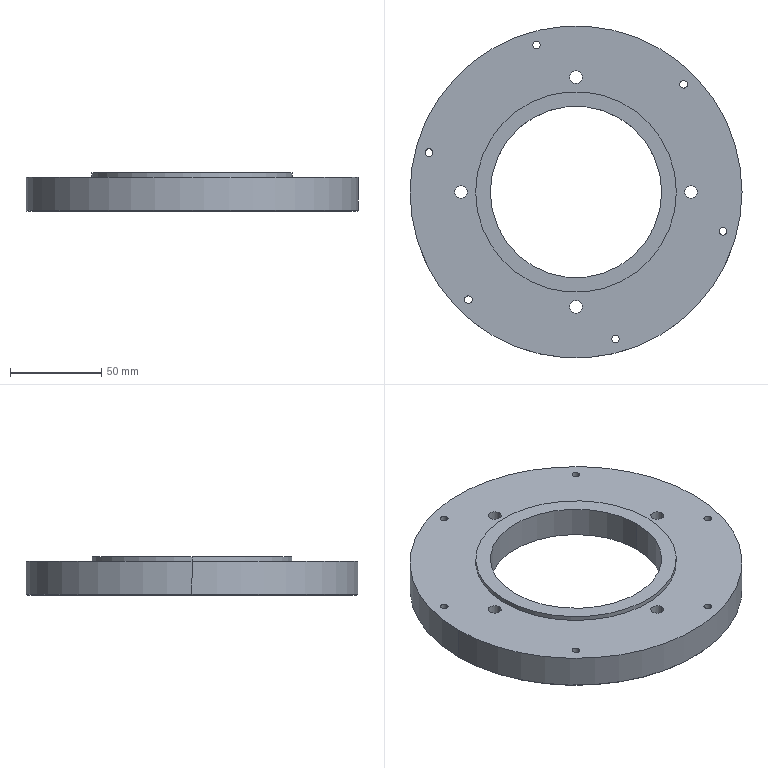Part | STEP file | Rear End Cover 2 | 1 solid | 46 faces | box 182 x 182 x 21 mm | volume 315087 mm3 | cylinder 36 | plane 8 | cone 2 | commonest cylinder face diameters 4.2 x12 7 x8 12 x8 94 x2 110 x2 145 x2
STEP:
#1=CARTESIAN_POINT('',(91.,0.,18.5));
#2=VERTEX_POINT('',#1);
#3=CARTESIAN_POINT('',(-91.,0.,18.5));
#4=VERTEX_POINT('',#3);
#5=CARTESIAN_POINT('',(0.,0.,18.5));
#6=DIRECTION('',(0.,0.,1.));
#7=DIRECTION('',(-1.,0.,0.));
#8=AXIS2_PLACEMENT_3D('',#5,#6,#7);
#9=CIRCLE('',#8,91.);
#10=EDGE_CURVE('',#2,#4,#9,.T.);
#11=ORIENTED_EDGE('',*,*,#10,.F.);
#12=CARTESIAN_POINT('',(91.,0.,0.5));
#13=VERTEX_POINT('',#12);
#14=CARTESIAN_POINT('',(91.,0.,275.887));
#15=DIRECTION('',(0.,0.,-1.));
#16=VECTOR('',#15,1000.);
#17=LINE('',#14,#16);
#18=EDGE_CURVE('',#2,#13,#17,.T.);
#19=ORIENTED_EDGE('',*,*,#18,.T.);
#20=CARTESIAN_POINT('',(-91.,0.,0.5));
#21=VERTEX_POINT('',#20);
#22=CARTESIAN_POINT('',(0.,0.,0.5));
#23=DIRECTION('',(0.,0.,1.));
#24=DIRECTION('',(-1.,0.,0.));
#25=AXIS2_PLACEMENT_3D('',#22,#23,#24);
#26=CIRCLE('',#25,91.);
#27=EDGE_CURVE('',#13,#21,#26,.T.);
#28=ORIENTED_EDGE('',*,*,#27,.T.);
#29=CARTESIAN_POINT('',(-91.,0.,275.887));
#30=DIRECTION('',(0.,0.,-1.));
#31=VECTOR('',#30,1000.);
#32=LINE('',#29,#31);
#33=EDGE_CURVE('',#4,#21,#32,.T.);
#34=ORIENTED_EDGE('',*,*,#33,.F.);
#35=EDGE_LOOP('',(#11,#19,#28,#34));
#36=FACE_OUTER_BOUND('',#35,.T.);
#37=CARTESIAN_POINT('',(0.,0.,275.887));
#38=DIRECTION('',(0.,0.,-1.));
#39=DIRECTION('',(-1.,0.,0.));
#40=AXIS2_PLACEMENT_3D('',#37,#38,#39);
#41=CYLINDRICAL_SURFACE('',#40,91.);
#42=ADVANCED_FACE('',(#36),#41,.T.);
#43=CARTESIAN_POINT('',(-55.,0.,21.));
#44=VERTEX_POINT('',#43);
#45=CARTESIAN_POINT('',(55.,0.,21.));
#46=VERTEX_POINT('',#45);
#47=CARTESIAN_POINT('',(0.,0.,21.));
#48=DIRECTION('',(0.,0.,-1.));
#49=DIRECTION('',(-1.,0.,0.));
#50=AXIS2_PLACEMENT_3D('',#47,#48,#49);
#51=CIRCLE('',#50,55.);
#52=EDGE_CURVE('',#44,#46,#51,.T.);
#53=ORIENTED_EDGE('',*,*,#52,.T.);
#54=CARTESIAN_POINT('',(55.,0.,18.5));
#55=VERTEX_POINT('',#54);
#56=CARTESIAN_POINT('',(55.,0.,21.));
#57=DIRECTION('',(0.,0.,-1.));
#58=VECTOR('',#57,1000.);
#59=LINE('',#56,#58);
#60=EDGE_CURVE('',#46,#55,#59,.T.);
#61=ORIENTED_EDGE('',*,*,#60,.T.);
#62=CARTESIAN_POINT('',(-55.,0.,18.5));
#63=VERTEX_POINT('',#62);
#64=CARTESIAN_POINT('',(0.,0.,18.5));
#65=DIRECTION('',(0.,0.,-1.));
#66=DIRECTION('',(-1.,0.,0.));
#67=AXIS2_PLACEMENT_3D('',#64,#65,#66);
#68=CIRCLE('',#67,55.);
#69=EDGE_CURVE('',#63,#55,#68,.T.);
#70=ORIENTED_EDGE('',*,*,#69,.F.);
#71=CARTESIAN_POINT('',(-55.,0.,21.));
#72=DIRECTION('',(0.,0.,-1.));
#73=VECTOR('',#72,1000.);
#74=LINE('',#71,#73);
#75=EDGE_CURVE('',#44,#63,#74,.T.);
#76=ORIENTED_EDGE('',*,*,#75,.F.);
#77=EDGE_LOOP('',(#53,#61,#70,#76));
#78=FACE_OUTER_BOUND('',#77,.T.);
#79=CARTESIAN_POINT('',(0.,0.,21.));
#80=DIRECTION('',(0.,0.,-1.));
#81=DIRECTION('',(-1.,0.,0.));
#82=AXIS2_PLACEMENT_3D('',#79,#80,#81);
#83=CYLINDRICAL_SURFACE('',#82,55.);
#84=ADVANCED_FACE('',(#78),#83,.T.);
#85=CARTESIAN_POINT('',(-3.5,63.,11.));
#86=VERTEX_POINT('',#85);
#87=CARTESIAN_POINT('',(3.5,63.,11.));
#88=VERTEX_POINT('',#87);
#89=CARTESIAN_POINT('',(0.,63.,11.));
#90=DIRECTION('',(0.,0.,1.));
#91=DIRECTION('',(1.,0.,0.));
#92=AXIS2_PLACEMENT_3D('',#89,#90,#91);
#93=CIRCLE('',#92,3.5);
#94=EDGE_CURVE('',#86,#88,#93,.T.);
#95=ORIENTED_EDGE('',*,*,#94,.F.);
#96=CARTESIAN_POINT('',(-3.5,63.,18.5));
#97=VERTEX_POINT('',#96);
#98=CARTESIAN_POINT('',(-3.5,63.,0.));
#99=DIRECTION('',(0.,0.,1.));
#100=VECTOR('',#99,1000.);
#101=LINE('',#98,#100);
#102=EDGE_CURVE('',#86,#97,#101,.T.);
#103=ORIENTED_EDGE('',*,*,#102,.T.);
#104=CARTESIAN_POINT('',(3.5,63.,18.5));
#105=VERTEX_POINT('',#104);
#106=CARTESIAN_POINT('',(0.,63.,18.5));
#107=DIRECTION('',(0.,0.,-1.));
#108=DIRECTION('',(1.,0.,0.));
#109=AXIS2_PLACEMENT_3D('',#106,#107,#108);
#110=CIRCLE('',#109,3.5);
#111=EDGE_CURVE('',#105,#97,#110,.T.);
#112=ORIENTED_EDGE('',*,*,#111,.F.);
#113=CARTESIAN_POINT('',(3.5,63.,0.));
#114=DIRECTION('',(0.,0.,1.));
#115=VECTOR('',#114,1000.);
#116=LINE('',#113,#115);
#117=EDGE_CURVE('',#88,#105,#116,.T.);
#118=ORIENTED_EDGE('',*,*,#117,.F.);
#119=EDGE_LOOP('',(#95,#103,#112,#118));
#120=FACE_OUTER_BOUND('',#119,.T.);
#121=CARTESIAN_POINT('',(0.,63.,0.));
#122=DIRECTION('',(0.,0.,1.));
#123=DIRECTION('',(1.,0.,0.));
#124=AXIS2_PLACEMENT_3D('',#121,#122,#123);
#125=CYLINDRICAL_SURFACE('',#124,3.5);
#126=ADVANCED_FACE('',(#120),#125,.F.);
#127=CARTESIAN_POINT('',(59.5,0.,11.));
#128=VERTEX_POINT('',#127);
#129=CARTESIAN_POINT('',(66.5,0.,11.));
#130=VERTEX_POINT('',#129);
#131=CARTESIAN_POINT('',(63.,0.,11.));
#132=DIRECTION('',(0.,0.,1.));
#133=DIRECTION('',(1.,0.,0.));
#134=AXIS2_PLACEMENT_3D('',#131,#132,#133);
#135=CIRCLE('',#134,3.5);
#136=EDGE_CURVE('',#128,#130,#135,.T.);
#137=ORIENTED_EDGE('',*,*,#136,.F.);
#138=CARTESIAN_POINT('',(59.5,0.,18.5));
#139=VERTEX_POINT('',#138);
#140=CARTESIAN_POINT('',(59.5,0.,0.));
#141=DIRECTION('',(0.,0.,1.));
#142=VECTOR('',#141,1000.);
#143=LINE('',#140,#142);
#144=EDGE_CURVE('',#128,#139,#143,.T.);
#145=ORIENTED_EDGE('',*,*,#144,.T.);
#146=CARTESIAN_POINT('',(66.5,0.,18.5));
#147=VERTEX_POINT('',#146);
#148=CARTESIAN_POINT('',(63.,0.,18.5));
#149=DIRECTION('',(0.,0.,-1.));
#150=DIRECTION('',(1.,0.,0.));
#151=AXIS2_PLACEMENT_3D('',#148,#149,#150);
#152=CIRCLE('',#151,3.5);
#153=EDGE_CURVE('',#147,#139,#152,.T.);
#154=ORIENTED_EDGE('',*,*,#153,.F.);
#155=CARTESIAN_POINT('',(66.5,0.,0.));
#156=DIRECTION('',(0.,0.,1.));
#157=VECTOR('',#156,1000.);
#158=LINE('',#155,#157);
#159=EDGE_CURVE('',#130,#147,#158,.T.);
#160=ORIENTED_EDGE('',*,*,#159,.F.);
#161=EDGE_LOOP('',(#137,#145,#154,#160));
#162=FACE_OUTER_BOUND('',#161,.T.);
#163=CARTESIAN_POINT('',(63.,0.,0.));
#164=DIRECTION('',(0.,0.,1.));
#165=DIRECTION('',(1.,0.,0.));
#166=AXIS2_PLACEMENT_3D('',#163,#164,#165);
#167=CYLINDRICAL_SURFACE('',#166,3.5);
#168=ADVANCED_FACE('',(#162),#167,.F.);
#169=CARTESIAN_POINT('',(-3.5,-63.,11.));
#170=VERTEX_POINT('',#169);
#171=CARTESIAN_POINT('',(3.5,-63.,11.));
#172=VERTEX_POINT('',#171);
#173=CARTESIAN_POINT('',(0.,-63.,11.));
#174=DIRECTION('',(0.,0.,1.));
#175=DIRECTION('',(1.,0.,0.));
#176=AXIS2_PLACEMENT_3D('',#173,#174,#175);
#177=CIRCLE('',#176,3.5);
#178=EDGE_CURVE('',#170,#172,#177,.T.);
#179=ORIENTED_EDGE('',*,*,#178,.F.);
#180=CARTESIAN_POINT('',(-3.5,-63.,18.5));
#181=VERTEX_POINT('',#180);
#182=CARTESIAN_POINT('',(-3.5,-63.,0.));
#183=DIRECTION('',(0.,0.,1.));
#184=VECTOR('',#183,1000.);
#185=LINE('',#182,#184);
#186=EDGE_CURVE('',#170,#181,#185,.T.);
#187=ORIENTED_EDGE('',*,*,#186,.T.);
#188=CARTESIAN_POINT('',(3.5,-63.,18.5));
#189=VERTEX_POINT('',#188);
#190=CARTESIAN_POINT('',(0.,-63.,18.5));
#191=DIRECTION('',(0.,0.,-1.));
#192=DIRECTION('',(1.,0.,0.));
#193=AXIS2_PLACEMENT_3D('',#190,#191,#192);
#194=CIRCLE('',#193,3.5);
#195=EDGE_CURVE('',#189,#181,#194,.T.);
#196=ORIENTED_EDGE('',*,*,#195,.F.);
#197=CARTESIAN_POINT('',(3.5,-63.,0.));
#198=DIRECTION('',(0.,0.,1.));
#199=VECTOR('',#198,1000.);
#200=LINE('',#197,#199);
#201=EDGE_CURVE('',#172,#189,#200,.T.);
#202=ORIENTED_EDGE('',*,*,#201,.F.);
#203=EDGE_LOOP('',(#179,#187,#196,#202));
#204=FACE_OUTER_BOUND('',#203,.T.);
#205=CARTESIAN_POINT('',(0.,-63.,0.));
#206=DIRECTION('',(0.,0.,1.));
#207=DIRECTION('',(1.,0.,0.));
#208=AXIS2_PLACEMENT_3D('',#205,#206,#207);
#209=CYLINDRICAL_SURFACE('',#208,3.5);
#210=ADVANCED_FACE('',(#204),#209,.F.);
#211=CARTESIAN_POINT('',(-66.5,0.,11.));
#212=VERTEX_POINT('',#211);
#213=CARTESIAN_POINT('',(-59.5,0.,11.));
#214=VERTEX_POINT('',#213);
#215=CARTESIAN_POINT('',(-63.,0.,11.));
#216=DIRECTION('',(0.,0.,1.));
#217=DIRECTION('',(1.,0.,0.));
#218=AXIS2_PLACEMENT_3D('',#215,#216,#217);
#219=CIRCLE('',#218,3.5);
#220=EDGE_CURVE('',#212,#214,#219,.T.);
#221=ORIENTED_EDGE('',*,*,#220,.F.);
#222=CARTESIAN_POINT('',(-66.5,0.,18.5));
#223=VERTEX_POINT('',#222);
#224=CARTESIAN_POINT('',(-66.5,0.,0.));
#225=DIRECTION('',(0.,0.,1.));
#226=VECTOR('',#225,1000.);
#227=LINE('',#224,#226);
#228=EDGE_CURVE('',#212,#223,#227,.T.);
#229=ORIENTED_EDGE('',*,*,#228,.T.);
#230=CARTESIAN_POINT('',(-59.5,0.,18.5));
#231=VERTEX_POINT('',#230);
#232=CARTESIAN_POINT('',(-63.,0.,18.5));
#233=DIRECTION('',(0.,0.,-1.));
#234=DIRECTION('',(1.,0.,0.));
#235=AXIS2_PLACEMENT_3D('',#232,#233,#234);
#236=CIRCLE('',#235,3.5);
#237=EDGE_CURVE('',#231,#223,#236,.T.);
#238=ORIENTED_EDGE('',*,*,#237,.F.);
#239=CARTESIAN_POINT('',(-59.5,0.,0.));
#240=DIRECTION('',(0.,0.,1.));
#241=VECTOR('',#240,1000.);
#242=LINE('',#239,#241);
#243=EDGE_CURVE('',#214,#231,#242,.T.);
#244=ORIENTED_EDGE('',*,*,#243,.F.);
#245=EDGE_LOOP('',(#221,#229,#238,#244));
#246=FACE_OUTER_BOUND('',#245,.T.);
#247=CARTESIAN_POINT('',(-63.,0.,0.));
#248=DIRECTION('',(0.,0.,1.));
#249=DIRECTION('',(1.,0.,0.));
#250=AXIS2_PLACEMENT_3D('',#247,#248,#249);
#251=CYLINDRICAL_SURFACE('',#250,3.5);
#252=ADVANCED_FACE('',(#246),#251,.F.);
#253=CARTESIAN_POINT('',(61.101,59.001,18.5));
#254=VERTEX_POINT('',#253);
#255=CARTESIAN_POINT('',(56.901,59.001,18.5));
#256=VERTEX_POINT('',#255);
#257=CARTESIAN_POINT('',(59.001,59.001,18.5));
#258=DIRECTION('',(0.,0.,-1.));
#259=DIRECTION('',(-1.,0.,0.));
#260=AXIS2_PLACEMENT_3D('',#257,#258,#259);
#261=CIRCLE('',#260,2.1);
#262=EDGE_CURVE('',#254,#256,#261,.T.);
#263=ORIENTED_EDGE('',*,*,#262,.F.);
#264=CARTESIAN_POINT('',(61.101,59.001,0.));
#265=VERTEX_POINT('',#264);
#266=CARTESIAN_POINT('',(61.101,59.001,21.));
#267=DIRECTION('',(0.,0.,-1.));
#268=VECTOR('',#267,1000.);
#269=LINE('',#266,#268);
#270=EDGE_CURVE('',#254,#265,#269,.T.);
#271=ORIENTED_EDGE('',*,*,#270,.T.);
#272=CARTESIAN_POINT('',(56.901,59.001,0.));
#273=VERTEX_POINT('',#272);
#274=CARTESIAN_POINT('',(59.001,59.001,0.));
#275=DIRECTION('',(0.,0.,1.));
#276=DIRECTION('',(-1.,0.,0.));
#277=AXIS2_PLACEMENT_3D('',#274,#275,#276);
#278=CIRCLE('',#277,2.1);
#279=EDGE_CURVE('',#273,#265,#278,.T.);
#280=ORIENTED_EDGE('',*,*,#279,.F.);
#281=CARTESIAN_POINT('',(56.901,59.001,21.));
#282=DIRECTION('',(0.,0.,-1.));
#283=VECTOR('',#282,1000.);
#284=LINE('',#281,#283);
#285=EDGE_CURVE('',#256,#273,#284,.T.);
#286=ORIENTED_EDGE('',*,*,#285,.F.);
#287=EDGE_LOOP('',(#263,#271,#280,#286));
#288=FACE_OUTER_BOUND('',#287,.T.);
#289=CARTESIAN_POINT('',(59.001,59.001,21.));
#290=DIRECTION('',(0.,0.,-1.));
#291=DIRECTION('',(-1.,0.,0.));
#292=AXIS2_PLACEMENT_3D('',#289,#290,#291);
#293=CYLINDRICAL_SURFACE('',#292,2.1);
#294=ADVANCED_FACE('',(#288),#293,.F.);
#295=CARTESIAN_POINT('',(-19.496,80.597,18.5));
#296=VERTEX_POINT('',#295);
#297=CARTESIAN_POINT('',(-23.696,80.597,18.5));
#298=VERTEX_POINT('',#297);
#299=CARTESIAN_POINT('',(-21.596,80.597,18.5));
#300=DIRECTION('',(0.,0.,-1.));
#301=DIRECTION('',(-1.,0.,0.));
#302=AXIS2_PLACEMENT_3D('',#299,#300,#301);
#303=CIRCLE('',#302,2.1);
#304=EDGE_CURVE('',#296,#298,#303,.T.);
#305=ORIENTED_EDGE('',*,*,#304,.F.);
#306=CARTESIAN_POINT('',(-19.496,80.597,0.));
#307=VERTEX_POINT('',#306);
#308=CARTESIAN_POINT('',(-19.496,80.597,21.));
#309=DIRECTION('',(0.,0.,-1.));
#310=VECTOR('',#309,1000.);
#311=LINE('',#308,#310);
#312=EDGE_CURVE('',#296,#307,#311,.T.);
#313=ORIENTED_EDGE('',*,*,#312,.T.);
#314=CARTESIAN_POINT('',(-23.696,80.597,0.));
#315=VERTEX_POINT('',#314);
#316=CARTESIAN_POINT('',(-21.596,80.597,0.));
#317=DIRECTION('',(0.,0.,1.));
#318=DIRECTION('',(-1.,0.,0.));
#319=AXIS2_PLACEMENT_3D('',#316,#317,#318);
#320=CIRCLE('',#319,2.1);
#321=EDGE_CURVE('',#315,#307,#320,.T.);
#322=ORIENTED_EDGE('',*,*,#321,.F.);
#323=CARTESIAN_POINT('',(-23.696,80.597,21.));
#324=DIRECTION('',(0.,0.,-1.));
#325=VECTOR('',#324,1000.);
#326=LINE('',#323,#325);
#327=EDGE_CURVE('',#298,#315,#326,.T.);
#328=ORIENTED_EDGE('',*,*,#327,.F.);
#329=EDGE_LOOP('',(#305,#313,#322,#328));
#330=FACE_OUTER_BOUND('',#329,.T.);
#331=CARTESIAN_POINT('',(-21.596,80.597,21.));
#332=DIRECTION('',(0.,0.,-1.));
#333=DIRECTION('',(-1.,0.,0.));
#334=AXIS2_PLACEMENT_3D('',#331,#332,#333);
#335=CYLINDRICAL_SURFACE('',#334,2.1);
#336=ADVANCED_FACE('',(#330),#335,.F.);
#337=CARTESIAN_POINT('',(-78.497,21.596,18.5));
#338=VERTEX_POINT('',#337);
#339=CARTESIAN_POINT('',(-82.697,21.596,18.5));
#340=VERTEX_POINT('',#339);
#341=CARTESIAN_POINT('',(-80.597,21.596,18.5));
#342=DIRECTION('',(0.,0.,-1.));
#343=DIRECTION('',(-1.,0.,0.));
#344=AXIS2_PLACEMENT_3D('',#341,#342,#343);
#345=CIRCLE('',#344,2.1);
#346=EDGE_CURVE('',#338,#340,#345,.T.);
#347=ORIENTED_EDGE('',*,*,#346,.F.);
#348=CARTESIAN_POINT('',(-78.497,21.596,0.));
#349=VERTEX_POINT('',#348);
#350=CARTESIAN_POINT('',(-78.497,21.596,21.));
#351=DIRECTION('',(0.,0.,-1.));
#352=VECTOR('',#351,1000.);
#353=LINE('',#350,#352);
#354=EDGE_CURVE('',#338,#349,#353,.T.);
#355=ORIENTED_EDGE('',*,*,#354,.T.);
#356=CARTESIAN_POINT('',(-82.697,21.596,0.));
#357=VERTEX_POINT('',#356);
#358=CARTESIAN_POINT('',(-80.597,21.596,0.));
#359=DIRECTION('',(0.,0.,1.));
#360=DIRECTION('',(-1.,0.,0.));
#361=AXIS2_PLACEMENT_3D('',#358,#359,#360);
#362=CIRCLE('',#361,2.1);
#363=EDGE_CURVE('',#357,#349,#362,.T.);
#364=ORIENTED_EDGE('',*,*,#363,.F.);
#365=CARTESIAN_POINT('',(-82.697,21.596,21.));
#366=DIRECTION('',(0.,0.,-1.));
#367=VECTOR('',#366,1000.);
#368=LINE('',#365,#367);
#369=EDGE_CURVE('',#340,#357,#368,.T.);
#370=ORIENTED_EDGE('',*,*,#369,.F.);
#371=EDGE_LOOP('',(#347,#355,#364,#370));
#372=FACE_OUTER_BOUND('',#371,.T.);
#373=CARTESIAN_POINT('',(-80.597,21.596,21.));
#374=DIRECTION('',(0.,0.,-1.));
#375=DIRECTION('',(-1.,0.,0.));
#376=AXIS2_PLACEMENT_3D('',#373,#374,#375);
#377=CYLINDRICAL_SURFACE('',#376,2.1);
#378=ADVANCED_FACE('',(#372),#377,.F.);
#379=CARTESIAN_POINT('',(-56.901,-59.001,18.5));
#380=VERTEX_POINT('',#379);
#381=CARTESIAN_POINT('',(-61.101,-59.001,18.5));
#382=VERTEX_POINT('',#381);
#383=CARTESIAN_POINT('',(-59.001,-59.001,18.5));
#384=DIRECTION('',(0.,0.,-1.));
#385=DIRECTION('',(-1.,0.,0.));
#386=AXIS2_PLACEMENT_3D('',#383,#384,#385);
#387=CIRCLE('',#386,2.1);
#388=EDGE_CURVE('',#380,#382,#387,.T.);
#389=ORIENTED_EDGE('',*,*,#388,.F.);
#390=CARTESIAN_POINT('',(-56.901,-59.001,0.));
#391=VERTEX_POINT('',#390);
#392=CARTESIAN_POINT('',(-56.901,-59.001,21.));
#393=DIRECTION('',(0.,0.,-1.));
#394=VECTOR('',#393,1000.);
#395=LINE('',#392,#394);
#396=EDGE_CURVE('',#380,#391,#395,.T.);
#397=ORIENTED_EDGE('',*,*,#396,.T.);
#398=CARTESIAN_POINT('',(-61.101,-59.001,0.));
#399=VERTEX_POINT('',#398);
#400=CARTESIAN_POINT('',(-59.001,-59.001,0.));
#401=DIRECTION('',(0.,0.,1.));
#402=DIRECTION('',(-1.,0.,0.));
#403=AXIS2_PLACEMENT_3D('',#400,#401,#402);
#404=CIRCLE('',#403,2.1);
#405=EDGE_CURVE('',#399,#391,#404,.T.);
#406=ORIENTED_EDGE('',*,*,#405,.F.);
#407=CARTESIAN_POINT('',(-61.101,-59.001,21.));
#408=DIRECTION('',(0.,0.,-1.));
#409=VECTOR('',#408,1000.);
#410=LINE('',#407,#409);
#411=EDGE_CURVE('',#382,#399,#410,.T.);
#412=ORIENTED_EDGE('',*,*,#411,.F.);
#413=EDGE_LOOP('',(#389,#397,#406,#412));
#414=FACE_OUTER_BOUND('',#413,.T.);
#415=CARTESIAN_POINT('',(-59.001,-59.001,21.));
#416=DIRECTION('',(0.,0.,-1.));
#417=DIRECTION('',(-1.,0.,0.));
#418=AXIS2_PLACEMENT_3D('',#415,#416,#417);
#419=CYLINDRICAL_SURFACE('',#418,2.1);
#420=ADVANCED_FACE('',(#414),#419,.F.);
#421=CARTESIAN_POINT('',(23.696,-80.597,18.5));
#422=VERTEX_POINT('',#421);
#423=CARTESIAN_POINT('',(19.496,-80.597,18.5));
#424=VERTEX_POINT('',#423);
#425=CARTESIAN_POINT('',(21.596,-80.597,18.5));
#426=DIRECTION('',(0.,0.,-1.));
#427=DIRECTION('',(-1.,0.,0.));
#428=AXIS2_PLACEMENT_3D('',#425,#426,#427);
#429=CIRCLE('',#428,2.1);
#430=EDGE_CURVE('',#422,#424,#429,.T.);
#431=ORIENTED_EDGE('',*,*,#430,.F.);
#432=CARTESIAN_POINT('',(23.696,-80.597,0.));
#433=VERTEX_POINT('',#432);
#434=CARTESIAN_POINT('',(23.696,-80.597,21.));
#435=DIRECTION('',(0.,0.,-1.));
#436=VECTOR('',#435,1000.);
#437=LINE('',#434,#436);
#438=EDGE_CURVE('',#422,#433,#437,.T.);
#439=ORIENTED_EDGE('',*,*,#438,.T.);
#440=CARTESIAN_POINT('',(19.496,-80.597,0.));
#441=VERTEX_POINT('',#440);
#442=CARTESIAN_POINT('',(21.596,-80.597,0.));
#443=DIRECTION('',(0.,0.,1.));
#444=DIRECTION('',(-1.,0.,0.));
#445=AXIS2_PLACEMENT_3D('',#442,#443,#444);
#446=CIRCLE('',#445,2.1);
#447=EDGE_CURVE('',#441,#433,#446,.T.);
#448=ORIENTED_EDGE('',*,*,#447,.F.);
#449=CARTESIAN_POINT('',(19.496,-80.597,21.));
#450=DIRECTION('',(0.,0.,-1.));
#451=VECTOR('',#450,1000.);
#452=LINE('',#449,#451);
#453=EDGE_CURVE('',#424,#441,#452,.T.);
#454=ORIENTED_EDGE('',*,*,#453,.F.);
#455=EDGE_LOOP('',(#431,#439,#448,#454));
#456=FACE_OUTER_BOUND('',#455,.T.);
#457=CARTESIAN_POINT('',(21.596,-80.597,21.));
#458=DIRECTION('',(0.,0.,-1.));
#459=DIRECTION('',(-1.,0.,0.));
#460=AXIS2_PLACEMENT_3D('',#457,#458,#459);
#461=CYLINDRICAL_SURFACE('',#460,2.1);
#462=ADVANCED_FACE('',(#456),#461,.F.);
#463=CARTESIAN_POINT('',(82.697,-21.596,18.5));
#464=VERTEX_POINT('',#463);
#465=CARTESIAN_POINT('',(78.497,-21.596,18.5));
#466=VERTEX_POINT('',#465);
#467=CARTESIAN_POINT('',(80.597,-21.596,18.5));
#468=DIRECTION('',(0.,0.,-1.));
#469=DIRECTION('',(-1.,0.,0.));
#470=AXIS2_PLACEMENT_3D('',#467,#468,#469);
#471=CIRCLE('',#470,2.1);
#472=EDGE_CURVE('',#464,#466,#471,.T.);
#473=ORIENTED_EDGE('',*,*,#472,.F.);
#474=CARTESIAN_POINT('',(82.697,-21.596,0.));
#475=VERTEX_POINT('',#474);
#476=CARTESIAN_POINT('',(82.697,-21.596,21.));
#477=DIRECTION('',(0.,0.,-1.));
#478=VECTOR('',#477,1000.);
#479=LINE('',#476,#478);
#480=EDGE_CURVE('',#464,#475,#479,.T.);
#481=ORIENTED_EDGE('',*,*,#480,.T.);
#482=CARTESIAN_POINT('',(78.497,-21.596,0.));
#483=VERTEX_POINT('',#482);
#484=CARTESIAN_POINT('',(80.597,-21.596,0.));
#485=DIRECTION('',(0.,0.,1.));
#486=DIRECTION('',(-1.,0.,0.));
#487=AXIS2_PLACEMENT_3D('',#484,#485,#486);
#488=CIRCLE('',#487,2.1);
#489=EDGE_CURVE('',#483,#475,#488,.T.);
#490=ORIENTED_EDGE('',*,*,#489,.F.);
#491=CARTESIAN_POINT('',(78.497,-21.596,21.));
#492=DIRECTION('',(0.,0.,-1.));
#493=VECTOR('',#492,1000.);
#494=LINE('',#491,#493);
#495=EDGE_CURVE('',#466,#483,#494,.T.);
#496=ORIENTED_EDGE('',*,*,#495,.F.);
#497=EDGE_LOOP('',(#473,#481,#490,#496));
#498=FACE_OUTER_BOUND('',#497,.T.);
#499=CARTESIAN_POINT('',(80.597,-21.596,21.));
#500=DIRECTION('',(0.,0.,-1.));
#501=DIRECTION('',(-1.,0.,0.));
#502=AXIS2_PLACEMENT_3D('',#499,#500,#501);
#503=CYLINDRICAL_SURFACE('',#502,2.1);
#504=ADVANCED_FACE('',(#498),#503,.F.);
#505=CARTESIAN_POINT('',(90.5,0.,0.));
#506=VERTEX_POINT('',#505);
#507=CARTESIAN_POINT('',(-90.5,0.,0.));
#508=VERTEX_POINT('',#507);
#509=CARTESIAN_POINT('',(0.,0.,0.));
#510=DIRECTION('',(0.,0.,1.));
#511=DIRECTION('',(1.,0.,0.));
#512=AXIS2_PLACEMENT_3D('',#509,#510,#511);
#513=CIRCLE('',#512,90.5);
#514=EDGE_CURVE('',#506,#508,#513,.T.);
#515=ORIENTED_EDGE('',*,*,#514,.T.);
#516=CARTESIAN_POINT('',(-91.,0.,0.5));
#517=DIRECTION('',(-0.7071,0.,0.7071));
#518=VECTOR('',#517,1000.);
#519=LINE('',#516,#518);
#520=EDGE_CURVE('',#508,#21,#519,.T.);
#521=ORIENTED_EDGE('',*,*,#520,.T.);
#522=ORIENTED_EDGE('',*,*,#27,.F.);
#523=CARTESIAN_POINT('',(91.,0.,0.5));
#524=DIRECTION('',(0.7071,0.,0.7071));
#525=VECTOR('',#524,1000.);
#526=LINE('',#523,#525);
#527=EDGE_CURVE('',#506,#13,#526,.T.);
#528=ORIENTED_EDGE('',*,*,#527,.F.);
#529=EDGE_LOOP('',(#515,#521,#522,#528));
#530=FACE_OUTER_BOUND('',#529,.T.);
#531=CARTESIAN_POINT('',(0.,0.,0.5));
#532=DIRECTION('',(0.,0.,1.));
#533=DIRECTION('',(1.,0.,0.));
#534=AXIS2_PLACEMENT_3D('',#531,#532,#533);
#535=CONICAL_SURFACE('',#534,91.,0.7854);
#536=ADVANCED_FACE('',(#530),#535,.T.);
#537=CARTESIAN_POINT('',(47.,0.,21.));
#538=VERTEX_POINT('',#537);
#539=CARTESIAN_POINT('',(-47.,0.,21.));
#540=VERTEX_POINT('',#539);
#541=CARTESIAN_POINT('',(0.,0.,21.));
#542=DIRECTION('',(0.,0.,-1.));
#543=DIRECTION('',(-1.,0.,0.));
#544=AXIS2_PLACEMENT_3D('',#541,#542,#543);
#545=CIRCLE('',#544,47.);
#546=EDGE_CURVE('',#538,#540,#545,.T.);
#547=ORIENTED_EDGE('',*,*,#546,.F.);
#548=CARTESIAN_POINT('',(47.,0.,4.));
#549=VERTEX_POINT('',#548);
#550=CARTESIAN_POINT('',(47.,0.,18.5));
#551=DIRECTION('',(0.,0.,-1.));
#552=VECTOR('',#551,1000.);
#553=LINE('',#550,#552);
#554=EDGE_CURVE('',#538,#549,#553,.T.);
#555=ORIENTED_EDGE('',*,*,#554,.T.);
#556=CARTESIAN_POINT('',(-47.,0.,4.));
#557=VERTEX_POINT('',#556);
#558=CARTESIAN_POINT('',(0.,0.,4.));
#559=DIRECTION('',(0.,0.,1.));
#560=DIRECTION('',(-1.,0.,0.));
#561=AXIS2_PLACEMENT_3D('',#558,#559,#560);
#562=CIRCLE('',#561,47.);
#563=EDGE_CURVE('',#557,#549,#562,.T.);
#564=ORIENTED_EDGE('',*,*,#563,.F.);
#565=CARTESIAN_POINT('',(-47.,0.,18.5));
#566=DIRECTION('',(0.,0.,-1.));
#567=VECTOR('',#566,1000.);
#568=LINE('',#565,#567);
#569=EDGE_CURVE('',#540,#557,#568,.T.);
#570=ORIENTED_EDGE('',*,*,#569,.F.);
#571=EDGE_LOOP('',(#547,#555,#564,#570));
#572=FACE_OUTER_BOUND('',#571,.T.);
#573=CARTESIAN_POINT('',(0.,0.,18.5));
#574=DIRECTION('',(0.,0.,-1.));
#575=DIRECTION('',(-1.,0.,0.));
#576=AXIS2_PLACEMENT_3D('',#573,#574,#575);
#577=CYLINDRICAL_SURFACE('',#576,47.);
#578=ADVANCED_FACE('',(#572),#577,.F.);
#579=CARTESIAN_POINT('',(6.,63.,11.));
#580=VERTEX_POINT('',#579);
#581=CARTESIAN_POINT('',(-6.,63.,11.));
#582=VERTEX_POINT('',#581);
#583=CARTESIAN_POINT('',(0.,63.,11.));
#584=DIRECTION('',(0.,0.,-1.));
#585=DIRECTION('',(-1.,0.,0.));
#586=AXIS2_PLACEMENT_3D('',#583,#584,#585);
#587=CIRCLE('',#586,6.);
#588=EDGE_CURVE('',#580,#582,#587,.T.);
#589=ORIENTED_EDGE('',*,*,#588,.F.);
#590=CARTESIAN_POINT('',(6.,63.,4.));
#591=VERTEX_POINT('',#590);
#592=CARTESIAN_POINT('',(6.,63.,11.));
#593=DIRECTION('',(0.,0.,-1.));
#594=VECTOR('',#593,1000.);
#595=LINE('',#592,#594);
#596=EDGE_CURVE('',#580,#591,#595,.T.);
#597=ORIENTED_EDGE('',*,*,#596,.T.);
#598=CARTESIAN_POINT('',(-6.,63.,4.));
#599=VERTEX_POINT('',#598);
#600=CARTESIAN_POINT('',(0.,63.,4.));
#601=DIRECTION('',(0.,0.,1.));
#602=DIRECTION('',(-1.,0.,0.));
#603=AXIS2_PLACEMENT_3D('',#600,#601,#602);
#604=CIRCLE('',#603,6.);
#605=EDGE_CURVE('',#599,#591,#604,.T.);
#606=ORIENTED_EDGE('',*,*,#605,.F.);
#607=CARTESIAN_POINT('',(-6.,63.,11.));
#608=DIRECTION('',(0.,0.,-1.));
#609=VECTOR('',#608,1000.);
#610=LINE('',#607,#609);
#611=EDGE_CURVE('',#582,#599,#610,.T.);
#612=ORIENTED_EDGE('',*,*,#611,.F.);
#613=EDGE_LOOP('',(#589,#597,#606,#612));
#614=FACE_OUTER_BOUND('',#613,.T.);
#615=CARTESIAN_POINT('',(0.,63.,11.));
#616=DIRECTION('',(0.,0.,-1.));
#617=DIRECTION('',(-1.,0.,0.));
#618=AXIS2_PLACEMENT_3D('',#615,#616,#617);
#619=CYLINDRICAL_SURFACE('',#618,6.);
#620=ADVANCED_FACE('',(#614),#619,.F.);
#621=CARTESIAN_POINT('',(69.,0.,11.));
#622=VERTEX_POINT('',#621);
#623=CARTESIAN_POINT('',(57.,0.,11.));
#624=VERTEX_POINT('',#623);
#625=CARTESIAN_POINT('',(63.,0.,11.));
#626=DIRECTION('',(0.,0.,-1.));
#627=DIRECTION('',(-1.,0.,0.));
#628=AXIS2_PLACEMENT_3D('',#625,#626,#627);
#629=CIRCLE('',#628,6.);
#630=EDGE_CURVE('',#622,#624,#629,.T.);
#631=ORIENTED_EDGE('',*,*,#630,.F.);
#632=CARTESIAN_POINT('',(69.,0.,4.));
#633=VERTEX_POINT('',#632);
#634=CARTESIAN_POINT('',(69.,0.,11.));
#635=DIRECTION('',(0.,0.,-1.));
#636=VECTOR('',#635,1000.);
#637=LINE('',#634,#636);
#638=EDGE_CURVE('',#622,#633,#637,.T.);
#639=ORIENTED_EDGE('',*,*,#638,.T.);
#640=CARTESIAN_POINT('',(57.,0.,4.));
#641=VERTEX_POINT('',#640);
#642=CARTESIAN_POINT('',(63.,0.,4.));
#643=DIRECTION('',(0.,0.,1.));
#644=DIRECTION('',(-1.,0.,0.));
#645=AXIS2_PLACEMENT_3D('',#642,#643,#644);
#646=CIRCLE('',#645,6.);
#647=EDGE_CURVE('',#641,#633,#646,.T.);
#648=ORIENTED_EDGE('',*,*,#647,.F.);
#649=CARTESIAN_POINT('',(57.,0.,11.));
#650=DIRECTION('',(0.,0.,-1.));
#651=VECTOR('',#650,1000.);
#652=LINE('',#649,#651);
#653=EDGE_CURVE('',#624,#641,#652,.T.);
#654=ORIENTED_EDGE('',*,*,#653,.F.);
#655=EDGE_LOOP('',(#631,#639,#648,#654));
#656=FACE_OUTER_BOUND('',#655,.T.);
#657=CARTESIAN_POINT('',(63.,0.,11.));
#658=DIRECTION('',(0.,0.,-1.));
#659=DIRECTION('',(-1.,0.,0.));
#660=AXIS2_PLACEMENT_3D('',#657,#658,#659);
#661=CYLINDRICAL_SURFACE('',#660,6.);
#662=ADVANCED_FACE('',(#656),#661,.F.);
#663=CARTESIAN_POINT('',(6.,-63.,11.));
#664=VERTEX_POINT('',#663);
#665=CARTESIAN_POINT('',(-6.,-63.,11.));
#666=VERTEX_POINT('',#665);
#667=CARTESIAN_POINT('',(0.,-63.,11.));
#668=DIRECTION('',(0.,0.,-1.));
#669=DIRECTION('',(-1.,0.,0.));
#670=AXIS2_PLACEMENT_3D('',#667,#668,#669);
#671=CIRCLE('',#670,6.);
#672=EDGE_CURVE('',#664,#666,#671,.T.);
#673=ORIENTED_EDGE('',*,*,#672,.F.);
#674=CARTESIAN_POINT('',(6.,-63.,4.));
#675=VERTEX_POINT('',#674);
#676=CARTESIAN_POINT('',(6.,-63.,11.));
#677=DIRECTION('',(0.,0.,-1.));
#678=VECTOR('',#677,1000.);
#679=LINE('',#676,#678);
#680=EDGE_CURVE('',#664,#675,#679,.T.);
#681=ORIENTED_EDGE('',*,*,#680,.T.);
#682=CARTESIAN_POINT('',(-6.,-63.,4.));
#683=VERTEX_POINT('',#682);
#684=CARTESIAN_POINT('',(0.,-63.,4.));
#685=DIRECTION('',(0.,0.,1.));
#686=DIRECTION('',(-1.,0.,0.));
#687=AXIS2_PLACEMENT_3D('',#684,#685,#686);
#688=CIRCLE('',#687,6.);
#689=EDGE_CURVE('',#683,#675,#688,.T.);
#690=ORIENTED_EDGE('',*,*,#689,.F.);
#691=CARTESIAN_POINT('',(-6.,-63.,11.));
#692=DIRECTION('',(0.,0.,-1.));
#693=VECTOR('',#692,1000.);
#694=LINE('',#691,#693);
#695=EDGE_CURVE('',#666,#683,#694,.T.);
#696=ORIENTED_EDGE('',*,*,#695,.F.);
#697=EDGE_LOOP('',(#673,#681,#690,#696));
#698=FACE_OUTER_BOUND('',#697,.T.);
#699=CARTESIAN_POINT('',(0.,-63.,11.));
#700=DIRECTION('',(0.,0.,-1.));
#701=DIRECTION('',(-1.,0.,0.));
#702=AXIS2_PLACEMENT_3D('',#699,#700,#701);
#703=CYLINDRICAL_SURFACE('',#702,6.);
#704=ADVANCED_FACE('',(#698),#703,.F.);
#705=CARTESIAN_POINT('',(-57.,0.,11.));
#706=VERTEX_POINT('',#705);
#707=CARTESIAN_POINT('',(-69.,0.,11.));
#708=VERTEX_POINT('',#707);
#709=CARTESIAN_POINT('',(-63.,0.,11.));
#710=DIRECTION('',(0.,0.,-1.));
#711=DIRECTION('',(-1.,0.,0.));
#712=AXIS2_PLACEMENT_3D('',#709,#710,#711);
#713=CIRCLE('',#712,6.);
#714=EDGE_CURVE('',#706,#708,#713,.T.);
#715=ORIENTED_EDGE('',*,*,#714,.F.);
#716=CARTESIAN_POINT('',(-57.,0.,4.));
#717=VERTEX_POINT('',#716);
#718=CARTESIAN_POINT('',(-57.,0.,11.));
#719=DIRECTION('',(0.,0.,-1.));
#720=VECTOR('',#719,1000.);
#721=LINE('',#718,#720);
#722=EDGE_CURVE('',#706,#717,#721,.T.);
#723=ORIENTED_EDGE('',*,*,#722,.T.);
#724=CARTESIAN_POINT('',(-69.,0.,4.));
#725=VERTEX_POINT('',#724);
#726=CARTESIAN_POINT('',(-63.,0.,4.));
#727=DIRECTION('',(0.,0.,1.));
#728=DIRECTION('',(-1.,0.,0.));
#729=AXIS2_PLACEMENT_3D('',#726,#727,#728);
#730=CIRCLE('',#729,6.);
#731=EDGE_CURVE('',#725,#717,#730,.T.);
#732=ORIENTED_EDGE('',*,*,#731,.F.);
#733=CARTESIAN_POINT('',(-69.,0.,11.));
#734=DIRECTION('',(0.,0.,-1.));
#735=VECTOR('',#734,1000.);
#736=LINE('',#733,#735);
#737=EDGE_CURVE('',#708,#725,#736,.T.);
#738=ORIENTED_EDGE('',*,*,#737,.F.);
#739=EDGE_LOOP('',(#715,#723,#732,#738));
#740=FACE_OUTER_BOUND('',#739,.T.);
#741=CARTESIAN_POINT('',(-63.,0.,11.));
#742=DIRECTION('',(0.,0.,-1.));
#743=DIRECTION('',(-1.,0.,0.));
#744=AXIS2_PLACEMENT_3D('',#741,#742,#743);
#745=CYLINDRICAL_SURFACE('',#744,6.);
#746=ADVANCED_FACE('',(#740),#745,.F.);
#747=CARTESIAN_POINT('',(72.5,0.,4.));
#748=VERTEX_POINT('',#747);
#749=CARTESIAN_POINT('',(-72.5,0.,4.));
#750=VERTEX_POINT('',#749);
#751=CARTESIAN_POINT('',(0.,0.,4.));
#752=DIRECTION('',(0.,0.,-1.));
#753=DIRECTION('',(-1.,0.,0.));
#754=AXIS2_PLACEMENT_3D('',#751,#752,#753);
#755=CIRCLE('',#754,72.5);
#756=EDGE_CURVE('',#748,#750,#755,.T.);
#757=ORIENTED_EDGE('',*,*,#756,.F.);
#758=CARTESIAN_POINT('',(72.5,0.,0.));
#759=VERTEX_POINT('',#758);
#760=CARTESIAN_POINT('',(72.5,0.,4.));
#761=DIRECTION('',(0.,0.,-1.));
#762=VECTOR('',#761,1000.);
#763=LINE('',#760,#762);
#764=EDGE_CURVE('',#748,#759,#763,.T.);
#765=ORIENTED_EDGE('',*,*,#764,.T.);
#766=CARTESIAN_POINT('',(-72.5,0.,0.));
#767=VERTEX_POINT('',#766);
#768=CARTESIAN_POINT('',(0.,0.,0.));
#769=DIRECTION('',(0.,0.,-1.));
#770=DIRECTION('',(-1.,0.,0.));
#771=AXIS2_PLACEMENT_3D('',#768,#769,#770);
#772=CIRCLE('',#771,72.5);
#773=EDGE_CURVE('',#759,#767,#772,.T.);
#774=ORIENTED_EDGE('',*,*,#773,.T.);
#775=CARTESIAN_POINT('',(-72.5,0.,4.));
#776=DIRECTION('',(0.,0.,-1.));
#777=VECTOR('',#776,1000.);
#778=LINE('',#775,#777);
#779=EDGE_CURVE('',#750,#767,#778,.T.);
#780=ORIENTED_EDGE('',*,*,#779,.F.);
#781=EDGE_LOOP('',(#757,#765,#774,#780));
#782=FACE_OUTER_BOUND('',#781,.T.);
#783=CARTESIAN_POINT('',(0.,0.,4.));
#784=DIRECTION('',(0.,0.,-1.));
#785=DIRECTION('',(-1.,0.,0.));
#786=AXIS2_PLACEMENT_3D('',#783,#784,#785);
#787=CYLINDRICAL_SURFACE('',#786,72.5);
#788=ADVANCED_FACE('',(#782),#787,.F.);
#789=CARTESIAN_POINT('',(0.,0.,18.5));
#790=DIRECTION('',(0.,0.,1.));
#791=DIRECTION('',(-1.,0.,0.));
#792=AXIS2_PLACEMENT_3D('',#789,#790,#791);
#793=CIRCLE('',#792,91.);
#794=EDGE_CURVE('',#4,#2,#793,.T.);
#795=ORIENTED_EDGE('',*,*,#794,.T.);
#796=ORIENTED_EDGE('',*,*,#10,.T.);
#797=EDGE_LOOP('',(#795,#796));
#798=FACE_OUTER_BOUND('',#797,.T.);
#799=ORIENTED_EDGE('',*,*,#69,.T.);
#800=CARTESIAN_POINT('',(0.,0.,18.5));
#801=DIRECTION('',(0.,0.,-1.));
#802=DIRECTION('',(-1.,0.,0.));
#803=AXIS2_PLACEMENT_3D('',#800,#801,#802);
#804=CIRCLE('',#803,55.);
#805=EDGE_CURVE('',#55,#63,#804,.T.);
#806=ORIENTED_EDGE('',*,*,#805,.T.);
#807=EDGE_LOOP('',(#799,#806));
#808=FACE_BOUND('',#807,.T.);
#809=ORIENTED_EDGE('',*,*,#111,.T.);
#810=CARTESIAN_POINT('',(0.,63.,18.5));
#811=DIRECTION('',(0.,0.,-1.));
#812=DIRECTION('',(1.,0.,0.));
#813=AXIS2_PLACEMENT_3D('',#810,#811,#812);
#814=CIRCLE('',#813,3.5);
#815=EDGE_CURVE('',#97,#105,#814,.T.);
#816=ORIENTED_EDGE('',*,*,#815,.T.);
#817=EDGE_LOOP('',(#809,#816));
#818=FACE_BOUND('',#817,.T.);
#819=ORIENTED_EDGE('',*,*,#153,.T.);
#820=CARTESIAN_POINT('',(63.,0.,18.5));
#821=DIRECTION('',(0.,0.,-1.));
#822=DIRECTION('',(1.,0.,0.));
#823=AXIS2_PLACEMENT_3D('',#820,#821,#822);
#824=CIRCLE('',#823,3.5);
#825=EDGE_CURVE('',#139,#147,#824,.T.);
#826=ORIENTED_EDGE('',*,*,#825,.T.);
#827=EDGE_LOOP('',(#819,#826));
#828=FACE_BOUND('',#827,.T.);
#829=ORIENTED_EDGE('',*,*,#195,.T.);
#830=CARTESIAN_POINT('',(0.,-63.,18.5));
#831=DIRECTION('',(0.,0.,-1.));
#832=DIRECTION('',(1.,0.,0.));
#833=AXIS2_PLACEMENT_3D('',#830,#831,#832);
#834=CIRCLE('',#833,3.5);
#835=EDGE_CURVE('',#181,#189,#834,.T.);
#836=ORIENTED_EDGE('',*,*,#835,.T.);
#837=EDGE_LOOP('',(#829,#836));
#838=FACE_BOUND('',#837,.T.);
#839=ORIENTED_EDGE('',*,*,#237,.T.);
#840=CARTESIAN_POINT('',(-63.,0.,18.5));
#841=DIRECTION('',(0.,0.,-1.));
#842=DIRECTION('',(1.,0.,0.));
#843=AXIS2_PLACEMENT_3D('',#840,#841,#842);
#844=CIRCLE('',#843,3.5);
#845=EDGE_CURVE('',#223,#231,#844,.T.);
#846=ORIENTED_EDGE('',*,*,#845,.T.);
#847=EDGE_LOOP('',(#839,#846));
#848=FACE_BOUND('',#847,.T.);
#849=CARTESIAN_POINT('',(59.001,59.001,18.5));
#850=DIRECTION('',(0.,0.,-1.));
#851=DIRECTION('',(-1.,0.,0.));
#852=AXIS2_PLACEMENT_3D('',#849,#850,#851);
#853=CIRCLE('',#852,2.1);
#854=EDGE_CURVE('',#256,#254,#853,.T.);
#855=ORIENTED_EDGE('',*,*,#854,.T.);
#856=ORIENTED_EDGE('',*,*,#262,.T.);
#857=EDGE_LOOP('',(#855,#856));
#858=FACE_BOUND('',#857,.T.);
#859=CARTESIAN_POINT('',(-21.596,80.597,18.5));
#860=DIRECTION('',(0.,0.,-1.));
#861=DIRECTION('',(-1.,0.,0.));
#862=AXIS2_PLACEMENT_3D('',#859,#860,#861);
#863=CIRCLE('',#862,2.1);
#864=EDGE_CURVE('',#298,#296,#863,.T.);
#865=ORIENTED_EDGE('',*,*,#864,.T.);
#866=ORIENTED_EDGE('',*,*,#304,.T.);
#867=EDGE_LOOP('',(#865,#866));
#868=FACE_BOUND('',#867,.T.);
#869=CARTESIAN_POINT('',(-80.597,21.596,18.5));
#870=DIRECTION('',(0.,0.,-1.));
#871=DIRECTION('',(-1.,0.,0.));
#872=AXIS2_PLACEMENT_3D('',#869,#870,#871);
#873=CIRCLE('',#872,2.1);
#874=EDGE_CURVE('',#340,#338,#873,.T.);
#875=ORIENTED_EDGE('',*,*,#874,.T.);
#876=ORIENTED_EDGE('',*,*,#346,.T.);
#877=EDGE_LOOP('',(#875,#876));
#878=FACE_BOUND('',#877,.T.);
#879=CARTESIAN_POINT('',(-59.001,-59.001,18.5));
#880=DIRECTION('',(0.,0.,-1.));
#881=DIRECTION('',(-1.,0.,0.));
#882=AXIS2_PLACEMENT_3D('',#879,#880,#881);
#883=CIRCLE('',#882,2.1);
#884=EDGE_CURVE('',#382,#380,#883,.T.);
#885=ORIENTED_EDGE('',*,*,#884,.T.);
#886=ORIENTED_EDGE('',*,*,#388,.T.);
#887=EDGE_LOOP('',(#885,#886));
#888=FACE_BOUND('',#887,.T.);
#889=CARTESIAN_POINT('',(21.596,-80.597,18.5));
#890=DIRECTION('',(0.,0.,-1.));
#891=DIRECTION('',(-1.,0.,0.));
#892=AXIS2_PLACEMENT_3D('',#889,#890,#891);
#893=CIRCLE('',#892,2.1);
#894=EDGE_CURVE('',#424,#422,#893,.T.);
#895=ORIENTED_EDGE('',*,*,#894,.T.);
#896=ORIENTED_EDGE('',*,*,#430,.T.);
#897=EDGE_LOOP('',(#895,#896));
#898=FACE_BOUND('',#897,.T.);
#899=CARTESIAN_POINT('',(80.597,-21.596,18.5));
#900=DIRECTION('',(0.,0.,-1.));
#901=DIRECTION('',(-1.,0.,0.));
#902=AXIS2_PLACEMENT_3D('',#899,#900,#901);
#903=CIRCLE('',#902,2.1);
#904=EDGE_CURVE('',#466,#464,#903,.T.);
#905=ORIENTED_EDGE('',*,*,#904,.T.);
#906=ORIENTED_EDGE('',*,*,#472,.T.);
#907=EDGE_LOOP('',(#905,#906));
#908=FACE_BOUND('',#907,.T.);
#909=CARTESIAN_POINT('',(0.,0.,18.5));
#910=DIRECTION('',(0.,0.,1.));
#911=DIRECTION('',(1.,0.,0.));
#912=AXIS2_PLACEMENT_3D('',#909,#910,#911);
#913=PLANE('',#912);
#914=ADVANCED_FACE('',(#798,#808,#818,#828,#838,#848,#858,#868,#878,#888,#898,#908),#913,.T.);
#915=ORIENTED_EDGE('',*,*,#18,.F.);
#916=ORIENTED_EDGE('',*,*,#794,.F.);
#917=ORIENTED_EDGE('',*,*,#33,.T.);
#918=CARTESIAN_POINT('',(0.,0.,0.5));
#919=DIRECTION('',(0.,0.,1.));
#920=DIRECTION('',(-1.,0.,0.));
#921=AXIS2_PLACEMENT_3D('',#918,#919,#920);
#922=CIRCLE('',#921,91.);
#923=EDGE_CURVE('',#21,#13,#922,.T.);
#924=ORIENTED_EDGE('',*,*,#923,.T.);
#925=EDGE_LOOP('',(#915,#916,#917,#924));
#926=FACE_OUTER_BOUND('',#925,.T.);
#927=CARTESIAN_POINT('',(0.,0.,275.887));
#928=DIRECTION('',(0.,0.,-1.));
#929=DIRECTION('',(-1.,0.,0.));
#930=AXIS2_PLACEMENT_3D('',#927,#928,#929);
#931=CYLINDRICAL_SURFACE('',#930,91.);
#932=ADVANCED_FACE('',(#926),#931,.T.);
#933=ORIENTED_EDGE('',*,*,#60,.F.);
#934=CARTESIAN_POINT('',(0.,0.,21.));
#935=DIRECTION('',(0.,0.,-1.));
#936=DIRECTION('',(-1.,0.,0.));
#937=AXIS2_PLACEMENT_3D('',#934,#935,#936);
#938=CIRCLE('',#937,55.);
#939=EDGE_CURVE('',#46,#44,#938,.T.);
#940=ORIENTED_EDGE('',*,*,#939,.T.);
#941=ORIENTED_EDGE('',*,*,#75,.T.);
#942=ORIENTED_EDGE('',*,*,#805,.F.);
#943=EDGE_LOOP('',(#933,#940,#941,#942));
#944=FACE_OUTER_BOUND('',#943,.T.);
#945=CARTESIAN_POINT('',(0.,0.,21.));
#946=DIRECTION('',(0.,0.,-1.));
#947=DIRECTION('',(-1.,0.,0.));
#948=AXIS2_PLACEMENT_3D('',#945,#946,#947);
#949=CYLINDRICAL_SURFACE('',#948,55.);
#950=ADVANCED_FACE('',(#944),#949,.T.);
#951=ORIENTED_EDGE('',*,*,#102,.F.);
#952=CARTESIAN_POINT('',(0.,63.,11.));
#953=DIRECTION('',(0.,0.,1.));
#954=DIRECTION('',(1.,0.,0.));
#955=AXIS2_PLACEMENT_3D('',#952,#953,#954);
#956=CIRCLE('',#955,3.5);
#957=EDGE_CURVE('',#88,#86,#956,.T.);
#958=ORIENTED_EDGE('',*,*,#957,.F.);
#959=ORIENTED_EDGE('',*,*,#117,.T.);
#960=ORIENTED_EDGE('',*,*,#815,.F.);
#961=EDGE_LOOP('',(#951,#958,#959,#960));
#962=FACE_OUTER_BOUND('',#961,.T.);
#963=CARTESIAN_POINT('',(0.,63.,0.));
#964=DIRECTION('',(0.,0.,1.));
#965=DIRECTION('',(1.,0.,0.));
#966=AXIS2_PLACEMENT_3D('',#963,#964,#965);
#967=CYLINDRICAL_SURFACE('',#966,3.5);
#968=ADVANCED_FACE('',(#962),#967,.F.);
#969=ORIENTED_EDGE('',*,*,#144,.F.);
#970=CARTESIAN_POINT('',(63.,0.,11.));
#971=DIRECTION('',(0.,0.,1.));
#972=DIRECTION('',(1.,0.,0.));
#973=AXIS2_PLACEMENT_3D('',#970,#971,#972);
#974=CIRCLE('',#973,3.5);
#975=EDGE_CURVE('',#130,#128,#974,.T.);
#976=ORIENTED_EDGE('',*,*,#975,.F.);
#977=ORIENTED_EDGE('',*,*,#159,.T.);
#978=ORIENTED_EDGE('',*,*,#825,.F.);
#979=EDGE_LOOP('',(#969,#976,#977,#978));
#980=FACE_OUTER_BOUND('',#979,.T.);
#981=CARTESIAN_POINT('',(63.,0.,0.));
#982=DIRECTION('',(0.,0.,1.));
#983=DIRECTION('',(1.,0.,0.));
#984=AXIS2_PLACEMENT_3D('',#981,#982,#983);
#985=CYLINDRICAL_SURFACE('',#984,3.5);
#986=ADVANCED_FACE('',(#980),#985,.F.);
#987=ORIENTED_EDGE('',*,*,#186,.F.);
#988=CARTESIAN_POINT('',(0.,-63.,11.));
#989=DIRECTION('',(0.,0.,1.));
#990=DIRECTION('',(1.,0.,0.));
#991=AXIS2_PLACEMENT_3D('',#988,#989,#990);
#992=CIRCLE('',#991,3.5);
#993=EDGE_CURVE('',#172,#170,#992,.T.);
#994=ORIENTED_EDGE('',*,*,#993,.F.);
#995=ORIENTED_EDGE('',*,*,#201,.T.);
#996=ORIENTED_EDGE('',*,*,#835,.F.);
#997=EDGE_LOOP('',(#987,#994,#995,#996));
#998=FACE_OUTER_BOUND('',#997,.T.);
#999=CARTESIAN_POINT('',(0.,-63.,0.));
#1000=DIRECTION('',(0.,0.,1.));
#1001=DIRECTION('',(1.,0.,0.));
#1002=AXIS2_PLACEMENT_3D('',#999,#1000,#1001);
#1003=CYLINDRICAL_SURFACE('',#1002,3.5);
#1004=ADVANCED_FACE('',(#998),#1003,.F.);
#1005=ORIENTED_EDGE('',*,*,#228,.F.);
#1006=CARTESIAN_POINT('',(-63.,0.,11.));
#1007=DIRECTION('',(0.,0.,1.));
#1008=DIRECTION('',(1.,0.,0.));
#1009=AXIS2_PLACEMENT_3D('',#1006,#1007,#1008);
#1010=CIRCLE('',#1009,3.5);
#1011=EDGE_CURVE('',#214,#212,#1010,.T.);
#1012=ORIENTED_EDGE('',*,*,#1011,.F.);
#1013=ORIENTED_EDGE('',*,*,#243,.T.);
#1014=ORIENTED_EDGE('',*,*,#845,.F.);
#1015=EDGE_LOOP('',(#1005,#1012,#1013,#1014));
#1016=FACE_OUTER_BOUND('',#1015,.T.);
#1017=CARTESIAN_POINT('',(-63.,0.,0.));
#1018=DIRECTION('',(0.,0.,1.));
#1019=DIRECTION('',(1.,0.,0.));
#1020=AXIS2_PLACEMENT_3D('',#1017,#1018,#1019);
#1021=CYLINDRICAL_SURFACE('',#1020,3.5);
#1022=ADVANCED_FACE('',(#1016),#1021,.F.);
#1023=ORIENTED_EDGE('',*,*,#270,.F.);
#1024=ORIENTED_EDGE('',*,*,#854,.F.);
#1025=ORIENTED_EDGE('',*,*,#285,.T.);
#1026=CARTESIAN_POINT('',(59.001,59.001,0.));
#1027=DIRECTION('',(0.,0.,1.));
#1028=DIRECTION('',(-1.,0.,0.));
#1029=AXIS2_PLACEMENT_3D('',#1026,#1027,#1028);
#1030=CIRCLE('',#1029,2.1);
#1031=EDGE_CURVE('',#265,#273,#1030,.T.);
#1032=ORIENTED_EDGE('',*,*,#1031,.F.);
#1033=EDGE_LOOP('',(#1023,#1024,#1025,#1032));
#1034=FACE_OUTER_BOUND('',#1033,.T.);
#1035=CARTESIAN_POINT('',(59.001,59.001,21.));
#1036=DIRECTION('',(0.,0.,-1.));
#1037=DIRECTION('',(-1.,0.,0.));
#1038=AXIS2_PLACEMENT_3D('',#1035,#1036,#1037);
#1039=CYLINDRICAL_SURFACE('',#1038,2.1);
#1040=ADVANCED_FACE('',(#1034),#1039,.F.);
#1041=ORIENTED_EDGE('',*,*,#312,.F.);
#1042=ORIENTED_EDGE('',*,*,#864,.F.);
#1043=ORIENTED_EDGE('',*,*,#327,.T.);
#1044=CARTESIAN_POINT('',(-21.596,80.597,0.));
#1045=DIRECTION('',(0.,0.,1.));
#1046=DIRECTION('',(-1.,0.,0.));
#1047=AXIS2_PLACEMENT_3D('',#1044,#1045,#1046);
#1048=CIRCLE('',#1047,2.1);
#1049=EDGE_CURVE('',#307,#315,#1048,.T.);
#1050=ORIENTED_EDGE('',*,*,#1049,.F.);
#1051=EDGE_LOOP('',(#1041,#1042,#1043,#1050));
#1052=FACE_OUTER_BOUND('',#1051,.T.);
#1053=CARTESIAN_POINT('',(-21.596,80.597,21.));
#1054=DIRECTION('',(0.,0.,-1.));
#1055=DIRECTION('',(-1.,0.,0.));
#1056=AXIS2_PLACEMENT_3D('',#1053,#1054,#1055);
#1057=CYLINDRICAL_SURFACE('',#1056,2.1);
#1058=ADVANCED_FACE('',(#1052),#1057,.F.);
#1059=ORIENTED_EDGE('',*,*,#354,.F.);
#1060=ORIENTED_EDGE('',*,*,#874,.F.);
#1061=ORIENTED_EDGE('',*,*,#369,.T.);
#1062=CARTESIAN_POINT('',(-80.597,21.596,0.));
#1063=DIRECTION('',(0.,0.,1.));
#1064=DIRECTION('',(-1.,0.,0.));
#1065=AXIS2_PLACEMENT_3D('',#1062,#1063,#1064);
#1066=CIRCLE('',#1065,2.1);
#1067=EDGE_CURVE('',#349,#357,#1066,.T.);
#1068=ORIENTED_EDGE('',*,*,#1067,.F.);
#1069=EDGE_LOOP('',(#1059,#1060,#1061,#1068));
#1070=FACE_OUTER_BOUND('',#1069,.T.);
#1071=CARTESIAN_POINT('',(-80.597,21.596,21.));
#1072=DIRECTION('',(0.,0.,-1.));
#1073=DIRECTION('',(-1.,0.,0.));
#1074=AXIS2_PLACEMENT_3D('',#1071,#1072,#1073);
#1075=CYLINDRICAL_SURFACE('',#1074,2.1);
#1076=ADVANCED_FACE('',(#1070),#1075,.F.);
#1077=ORIENTED_EDGE('',*,*,#396,.F.);
#1078=ORIENTED_EDGE('',*,*,#884,.F.);
#1079=ORIENTED_EDGE('',*,*,#411,.T.);
#1080=CARTESIAN_POINT('',(-59.001,-59.001,0.));
#1081=DIRECTION('',(0.,0.,1.));
#1082=DIRECTION('',(-1.,0.,0.));
#1083=AXIS2_PLACEMENT_3D('',#1080,#1081,#1082);
#1084=CIRCLE('',#1083,2.1);
#1085=EDGE_CURVE('',#391,#399,#1084,.T.);
#1086=ORIENTED_EDGE('',*,*,#1085,.F.);
#1087=EDGE_LOOP('',(#1077,#1078,#1079,#1086));
#1088=FACE_OUTER_BOUND('',#1087,.T.);
#1089=CARTESIAN_POINT('',(-59.001,-59.001,21.));
#1090=DIRECTION('',(0.,0.,-1.));
#1091=DIRECTION('',(-1.,0.,0.));
#1092=AXIS2_PLACEMENT_3D('',#1089,#1090,#1091);
#1093=CYLINDRICAL_SURFACE('',#1092,2.1);
#1094=ADVANCED_FACE('',(#1088),#1093,.F.);
#1095=ORIENTED_EDGE('',*,*,#438,.F.);
#1096=ORIENTED_EDGE('',*,*,#894,.F.);
#1097=ORIENTED_EDGE('',*,*,#453,.T.);
#1098=CARTESIAN_POINT('',(21.596,-80.597,0.));
#1099=DIRECTION('',(0.,0.,1.));
#1100=DIRECTION('',(-1.,0.,0.));
#1101=AXIS2_PLACEMENT_3D('',#1098,#1099,#1100);
#1102=CIRCLE('',#1101,2.1);
#1103=EDGE_CURVE('',#433,#441,#1102,.T.);
#1104=ORIENTED_EDGE('',*,*,#1103,.F.);
#1105=EDGE_LOOP('',(#1095,#1096,#1097,#1104));
#1106=FACE_OUTER_BOUND('',#1105,.T.);
#1107=CARTESIAN_POINT('',(21.596,-80.597,21.));
#1108=DIRECTION('',(0.,0.,-1.));
#1109=DIRECTION('',(-1.,0.,0.));
#1110=AXIS2_PLACEMENT_3D('',#1107,#1108,#1109);
#1111=CYLINDRICAL_SURFACE('',#1110,2.1);
#1112=ADVANCED_FACE('',(#1106),#1111,.F.);
#1113=ORIENTED_EDGE('',*,*,#480,.F.);
#1114=ORIENTED_EDGE('',*,*,#904,.F.);
#1115=ORIENTED_EDGE('',*,*,#495,.T.);
#1116=CARTESIAN_POINT('',(80.597,-21.596,0.));
#1117=DIRECTION('',(0.,0.,1.));
#1118=DIRECTION('',(-1.,0.,0.));
#1119=AXIS2_PLACEMENT_3D('',#1116,#1117,#1118);
#1120=CIRCLE('',#1119,2.1);
#1121=EDGE_CURVE('',#475,#483,#1120,.T.);
#1122=ORIENTED_EDGE('',*,*,#1121,.F.);
#1123=EDGE_LOOP('',(#1113,#1114,#1115,#1122));
#1124=FACE_OUTER_BOUND('',#1123,.T.);
#1125=CARTESIAN_POINT('',(80.597,-21.596,21.));
#1126=DIRECTION('',(0.,0.,-1.));
#1127=DIRECTION('',(-1.,0.,0.));
#1128=AXIS2_PLACEMENT_3D('',#1125,#1126,#1127);
#1129=CYLINDRICAL_SURFACE('',#1128,2.1);
#1130=ADVANCED_FACE('',(#1124),#1129,.F.);
#1131=ORIENTED_EDGE('',*,*,#520,.F.);
#1132=CARTESIAN_POINT('',(0.,0.,0.));
#1133=DIRECTION('',(0.,0.,1.));
#1134=DIRECTION('',(1.,0.,0.));
#1135=AXIS2_PLACEMENT_3D('',#1132,#1133,#1134);
#1136=CIRCLE('',#1135,90.5);
#1137=EDGE_CURVE('',#508,#506,#1136,.T.);
#1138=ORIENTED_EDGE('',*,*,#1137,.T.);
#1139=ORIENTED_EDGE('',*,*,#527,.T.);
#1140=ORIENTED_EDGE('',*,*,#923,.F.);
#1141=EDGE_LOOP('',(#1131,#1138,#1139,#1140));
#1142=FACE_OUTER_BOUND('',#1141,.T.);
#1143=CARTESIAN_POINT('',(0.,0.,0.5));
#1144=DIRECTION('',(0.,0.,1.));
#1145=DIRECTION('',(1.,0.,0.));
#1146=AXIS2_PLACEMENT_3D('',#1143,#1144,#1145);
#1147=CONICAL_SURFACE('',#1146,91.,0.7854);
#1148=ADVANCED_FACE('',(#1142),#1147,.T.);
#1149=CARTESIAN_POINT('',(0.,0.,21.));
#1150=DIRECTION('',(0.,0.,-1.));
#1151=DIRECTION('',(-1.,0.,0.));
#1152=AXIS2_PLACEMENT_3D('',#1149,#1150,#1151);
#1153=CIRCLE('',#1152,47.);
#1154=EDGE_CURVE('',#540,#538,#1153,.T.);
#1155=ORIENTED_EDGE('',*,*,#1154,.T.);
#1156=ORIENTED_EDGE('',*,*,#546,.T.);
#1157=EDGE_LOOP('',(#1155,#1156));
#1158=FACE_BOUND('',#1157,.T.);
#1159=ORIENTED_EDGE('',*,*,#52,.F.);
#1160=ORIENTED_EDGE('',*,*,#939,.F.);
#1161=EDGE_LOOP('',(#1159,#1160));
#1162=FACE_OUTER_BOUND('',#1161,.T.);
#1163=CARTESIAN_POINT('',(0.,0.,21.));
#1164=DIRECTION('',(0.,0.,1.));
#1165=DIRECTION('',(1.,0.,0.));
#1166=AXIS2_PLACEMENT_3D('',#1163,#1164,#1165);
#1167=PLANE('',#1166);
#1168=ADVANCED_FACE('',(#1158,#1162),#1167,.T.);
#1169=ORIENTED_EDGE('',*,*,#957,.T.);
#1170=ORIENTED_EDGE('',*,*,#94,.T.);
#1171=EDGE_LOOP('',(#1169,#1170));
#1172=FACE_BOUND('',#1171,.T.);
#1173=CARTESIAN_POINT('',(0.,63.,11.));
#1174=DIRECTION('',(0.,0.,-1.));
#1175=DIRECTION('',(-1.,0.,0.));
#1176=AXIS2_PLACEMENT_3D('',#1173,#1174,#1175);
#1177=CIRCLE('',#1176,6.);
#1178=EDGE_CURVE('',#582,#580,#1177,.T.);
#1179=ORIENTED_EDGE('',*,*,#1178,.T.);
#1180=ORIENTED_EDGE('',*,*,#588,.T.);
#1181=EDGE_LOOP('',(#1179,#1180));
#1182=FACE_OUTER_BOUND('',#1181,.T.);
#1183=CARTESIAN_POINT('',(0.,63.,11.));
#1184=DIRECTION('',(0.,0.,-1.));
#1185=DIRECTION('',(-1.,0.,0.));
#1186=AXIS2_PLACEMENT_3D('',#1183,#1184,#1185);
#1187=PLANE('',#1186);
#1188=ADVANCED_FACE('',(#1172,#1182),#1187,.T.);
#1189=ORIENTED_EDGE('',*,*,#975,.T.);
#1190=ORIENTED_EDGE('',*,*,#136,.T.);
#1191=EDGE_LOOP('',(#1189,#1190));
#1192=FACE_BOUND('',#1191,.T.);
#1193=CARTESIAN_POINT('',(63.,0.,11.));
#1194=DIRECTION('',(0.,0.,-1.));
#1195=DIRECTION('',(-1.,0.,0.));
#1196=AXIS2_PLACEMENT_3D('',#1193,#1194,#1195);
#1197=CIRCLE('',#1196,6.);
#1198=EDGE_CURVE('',#624,#622,#1197,.T.);
#1199=ORIENTED_EDGE('',*,*,#1198,.T.);
#1200=ORIENTED_EDGE('',*,*,#630,.T.);
#1201=EDGE_LOOP('',(#1199,#1200));
#1202=FACE_OUTER_BOUND('',#1201,.T.);
#1203=CARTESIAN_POINT('',(63.,0.,11.));
#1204=DIRECTION('',(0.,0.,-1.));
#1205=DIRECTION('',(-1.,0.,0.));
#1206=AXIS2_PLACEMENT_3D('',#1203,#1204,#1205);
#1207=PLANE('',#1206);
#1208=ADVANCED_FACE('',(#1192,#1202),#1207,.T.);
#1209=ORIENTED_EDGE('',*,*,#993,.T.);
#1210=ORIENTED_EDGE('',*,*,#178,.T.);
#1211=EDGE_LOOP('',(#1209,#1210));
#1212=FACE_BOUND('',#1211,.T.);
#1213=CARTESIAN_POINT('',(0.,-63.,11.));
#1214=DIRECTION('',(0.,0.,-1.));
#1215=DIRECTION('',(-1.,0.,0.));
#1216=AXIS2_PLACEMENT_3D('',#1213,#1214,#1215);
#1217=CIRCLE('',#1216,6.);
#1218=EDGE_CURVE('',#666,#664,#1217,.T.);
#1219=ORIENTED_EDGE('',*,*,#1218,.T.);
#1220=ORIENTED_EDGE('',*,*,#672,.T.);
#1221=EDGE_LOOP('',(#1219,#1220));
#1222=FACE_OUTER_BOUND('',#1221,.T.);
#1223=CARTESIAN_POINT('',(0.,-63.,11.));
#1224=DIRECTION('',(0.,0.,-1.));
#1225=DIRECTION('',(-1.,0.,0.));
#1226=AXIS2_PLACEMENT_3D('',#1223,#1224,#1225);
#1227=PLANE('',#1226);
#1228=ADVANCED_FACE('',(#1212,#1222),#1227,.T.);
#1229=ORIENTED_EDGE('',*,*,#1011,.T.);
#1230=ORIENTED_EDGE('',*,*,#220,.T.);
#1231=EDGE_LOOP('',(#1229,#1230));
#1232=FACE_BOUND('',#1231,.T.);
#1233=CARTESIAN_POINT('',(-63.,0.,11.));
#1234=DIRECTION('',(0.,0.,-1.));
#1235=DIRECTION('',(-1.,0.,0.));
#1236=AXIS2_PLACEMENT_3D('',#1233,#1234,#1235);
#1237=CIRCLE('',#1236,6.);
#1238=EDGE_CURVE('',#708,#706,#1237,.T.);
#1239=ORIENTED_EDGE('',*,*,#1238,.T.);
#1240=ORIENTED_EDGE('',*,*,#714,.T.);
#1241=EDGE_LOOP('',(#1239,#1240));
#1242=FACE_OUTER_BOUND('',#1241,.T.);
#1243=CARTESIAN_POINT('',(-63.,0.,11.));
#1244=DIRECTION('',(0.,0.,-1.));
#1245=DIRECTION('',(-1.,0.,0.));
#1246=AXIS2_PLACEMENT_3D('',#1243,#1244,#1245);
#1247=PLANE('',#1246);
#1248=ADVANCED_FACE('',(#1232,#1242),#1247,.T.);
#1249=ORIENTED_EDGE('',*,*,#279,.T.);
#1250=ORIENTED_EDGE('',*,*,#1031,.T.);
#1251=EDGE_LOOP('',(#1249,#1250));
#1252=FACE_BOUND('',#1251,.T.);
#1253=ORIENTED_EDGE('',*,*,#321,.T.);
#1254=ORIENTED_EDGE('',*,*,#1049,.T.);
#1255=EDGE_LOOP('',(#1253,#1254));
#1256=FACE_BOUND('',#1255,.T.);
#1257=ORIENTED_EDGE('',*,*,#363,.T.);
#1258=ORIENTED_EDGE('',*,*,#1067,.T.);
#1259=EDGE_LOOP('',(#1257,#1258));
#1260=FACE_BOUND('',#1259,.T.);
#1261=ORIENTED_EDGE('',*,*,#405,.T.);
#1262=ORIENTED_EDGE('',*,*,#1085,.T.);
#1263=EDGE_LOOP('',(#1261,#1262));
#1264=FACE_BOUND('',#1263,.T.);
#1265=ORIENTED_EDGE('',*,*,#447,.T.);
#1266=ORIENTED_EDGE('',*,*,#1103,.T.);
#1267=EDGE_LOOP('',(#1265,#1266));
#1268=FACE_BOUND('',#1267,.T.);
#1269=ORIENTED_EDGE('',*,*,#489,.T.);
#1270=ORIENTED_EDGE('',*,*,#1121,.T.);
#1271=EDGE_LOOP('',(#1269,#1270));
#1272=FACE_BOUND('',#1271,.T.);
#1273=ORIENTED_EDGE('',*,*,#514,.F.);
#1274=ORIENTED_EDGE('',*,*,#1137,.F.);
#1275=EDGE_LOOP('',(#1273,#1274));
#1276=FACE_OUTER_BOUND('',#1275,.T.);
#1277=CARTESIAN_POINT('',(0.,0.,0.));
#1278=DIRECTION('',(0.,0.,-1.));
#1279=DIRECTION('',(-1.,0.,0.));
#1280=AXIS2_PLACEMENT_3D('',#1277,#1278,#1279);
#1281=CIRCLE('',#1280,72.5);
#1282=EDGE_CURVE('',#767,#759,#1281,.T.);
#1283=ORIENTED_EDGE('',*,*,#1282,.F.);
#1284=ORIENTED_EDGE('',*,*,#773,.F.);
#1285=EDGE_LOOP('',(#1283,#1284));
#1286=FACE_BOUND('',#1285,.T.);
#1287=CARTESIAN_POINT('',(0.,0.,0.));
#1288=DIRECTION('',(0.,0.,1.));
#1289=DIRECTION('',(1.,0.,0.));
#1290=AXIS2_PLACEMENT_3D('',#1287,#1288,#1289);
#1291=PLANE('',#1290);
#1292=ADVANCED_FACE('',(#1252,#1256,#1260,#1264,#1268,#1272,#1276,#1286),#1291,.F.);
#1293=ORIENTED_EDGE('',*,*,#554,.F.);
#1294=ORIENTED_EDGE('',*,*,#1154,.F.);
#1295=ORIENTED_EDGE('',*,*,#569,.T.);
#1296=CARTESIAN_POINT('',(0.,0.,4.));
#1297=DIRECTION('',(0.,0.,1.));
#1298=DIRECTION('',(-1.,0.,0.));
#1299=AXIS2_PLACEMENT_3D('',#1296,#1297,#1298);
#1300=CIRCLE('',#1299,47.);
#1301=EDGE_CURVE('',#549,#557,#1300,.T.);
#1302=ORIENTED_EDGE('',*,*,#1301,.F.);
#1303=EDGE_LOOP('',(#1293,#1294,#1295,#1302));
#1304=FACE_OUTER_BOUND('',#1303,.T.);
#1305=CARTESIAN_POINT('',(0.,0.,18.5));
#1306=DIRECTION('',(0.,0.,-1.));
#1307=DIRECTION('',(-1.,0.,0.));
#1308=AXIS2_PLACEMENT_3D('',#1305,#1306,#1307);
#1309=CYLINDRICAL_SURFACE('',#1308,47.);
#1310=ADVANCED_FACE('',(#1304),#1309,.F.);
#1311=ORIENTED_EDGE('',*,*,#596,.F.);
#1312=ORIENTED_EDGE('',*,*,#1178,.F.);
#1313=ORIENTED_EDGE('',*,*,#611,.T.);
#1314=CARTESIAN_POINT('',(0.,63.,4.));
#1315=DIRECTION('',(0.,0.,1.));
#1316=DIRECTION('',(-1.,0.,0.));
#1317=AXIS2_PLACEMENT_3D('',#1314,#1315,#1316);
#1318=CIRCLE('',#1317,6.);
#1319=EDGE_CURVE('',#591,#599,#1318,.T.);
#1320=ORIENTED_EDGE('',*,*,#1319,.F.);
#1321=EDGE_LOOP('',(#1311,#1312,#1313,#1320));
#1322=FACE_OUTER_BOUND('',#1321,.T.);
#1323=CARTESIAN_POINT('',(0.,63.,11.));
#1324=DIRECTION('',(0.,0.,-1.));
#1325=DIRECTION('',(-1.,0.,0.));
#1326=AXIS2_PLACEMENT_3D('',#1323,#1324,#1325);
#1327=CYLINDRICAL_SURFACE('',#1326,6.);
#1328=ADVANCED_FACE('',(#1322),#1327,.F.);
#1329=ORIENTED_EDGE('',*,*,#638,.F.);
#1330=ORIENTED_EDGE('',*,*,#1198,.F.);
#1331=ORIENTED_EDGE('',*,*,#653,.T.);
#1332=CARTESIAN_POINT('',(63.,0.,4.));
#1333=DIRECTION('',(0.,0.,1.));
#1334=DIRECTION('',(-1.,0.,0.));
#1335=AXIS2_PLACEMENT_3D('',#1332,#1333,#1334);
#1336=CIRCLE('',#1335,6.);
#1337=EDGE_CURVE('',#633,#641,#1336,.T.);
#1338=ORIENTED_EDGE('',*,*,#1337,.F.);
#1339=EDGE_LOOP('',(#1329,#1330,#1331,#1338));
#1340=FACE_OUTER_BOUND('',#1339,.T.);
#1341=CARTESIAN_POINT('',(63.,0.,11.));
#1342=DIRECTION('',(0.,0.,-1.));
#1343=DIRECTION('',(-1.,0.,0.));
#1344=AXIS2_PLACEMENT_3D('',#1341,#1342,#1343);
#1345=CYLINDRICAL_SURFACE('',#1344,6.);
#1346=ADVANCED_FACE('',(#1340),#1345,.F.);
#1347=ORIENTED_EDGE('',*,*,#680,.F.);
#1348=ORIENTED_EDGE('',*,*,#1218,.F.);
#1349=ORIENTED_EDGE('',*,*,#695,.T.);
#1350=CARTESIAN_POINT('',(0.,-63.,4.));
#1351=DIRECTION('',(0.,0.,1.));
#1352=DIRECTION('',(-1.,0.,0.));
#1353=AXIS2_PLACEMENT_3D('',#1350,#1351,#1352);
#1354=CIRCLE('',#1353,6.);
#1355=EDGE_CURVE('',#675,#683,#1354,.T.);
#1356=ORIENTED_EDGE('',*,*,#1355,.F.);
#1357=EDGE_LOOP('',(#1347,#1348,#1349,#1356));
#1358=FACE_OUTER_BOUND('',#1357,.T.);
#1359=CARTESIAN_POINT('',(0.,-63.,11.));
#1360=DIRECTION('',(0.,0.,-1.));
#1361=DIRECTION('',(-1.,0.,0.));
#1362=AXIS2_PLACEMENT_3D('',#1359,#1360,#1361);
#1363=CYLINDRICAL_SURFACE('',#1362,6.);
#1364=ADVANCED_FACE('',(#1358),#1363,.F.);
#1365=ORIENTED_EDGE('',*,*,#722,.F.);
#1366=ORIENTED_EDGE('',*,*,#1238,.F.);
#1367=ORIENTED_EDGE('',*,*,#737,.T.);
#1368=CARTESIAN_POINT('',(-63.,0.,4.));
#1369=DIRECTION('',(0.,0.,1.));
#1370=DIRECTION('',(-1.,0.,0.));
#1371=AXIS2_PLACEMENT_3D('',#1368,#1369,#1370);
#1372=CIRCLE('',#1371,6.);
#1373=EDGE_CURVE('',#717,#725,#1372,.T.);
#1374=ORIENTED_EDGE('',*,*,#1373,.F.);
#1375=EDGE_LOOP('',(#1365,#1366,#1367,#1374));
#1376=FACE_OUTER_BOUND('',#1375,.T.);
#1377=CARTESIAN_POINT('',(-63.,0.,11.));
#1378=DIRECTION('',(0.,0.,-1.));
#1379=DIRECTION('',(-1.,0.,0.));
#1380=AXIS2_PLACEMENT_3D('',#1377,#1378,#1379);
#1381=CYLINDRICAL_SURFACE('',#1380,6.);
#1382=ADVANCED_FACE('',(#1376),#1381,.F.);
#1383=ORIENTED_EDGE('',*,*,#764,.F.);
#1384=CARTESIAN_POINT('',(0.,0.,4.));
#1385=DIRECTION('',(0.,0.,-1.));
#1386=DIRECTION('',(-1.,0.,0.));
#1387=AXIS2_PLACEMENT_3D('',#1384,#1385,#1386);
#1388=CIRCLE('',#1387,72.5);
#1389=EDGE_CURVE('',#750,#748,#1388,.T.);
#1390=ORIENTED_EDGE('',*,*,#1389,.F.);
#1391=ORIENTED_EDGE('',*,*,#779,.T.);
#1392=ORIENTED_EDGE('',*,*,#1282,.T.);
#1393=EDGE_LOOP('',(#1383,#1390,#1391,#1392));
#1394=FACE_OUTER_BOUND('',#1393,.T.);
#1395=CARTESIAN_POINT('',(0.,0.,4.));
#1396=DIRECTION('',(0.,0.,-1.));
#1397=DIRECTION('',(-1.,0.,0.));
#1398=AXIS2_PLACEMENT_3D('',#1395,#1396,#1397);
#1399=CYLINDRICAL_SURFACE('',#1398,72.5);
#1400=ADVANCED_FACE('',(#1394),#1399,.F.);
#1401=ORIENTED_EDGE('',*,*,#647,.T.);
#1402=ORIENTED_EDGE('',*,*,#1337,.T.);
#1403=EDGE_LOOP('',(#1401,#1402));
#1404=FACE_BOUND('',#1403,.T.);
#1405=ORIENTED_EDGE('',*,*,#731,.T.);
#1406=ORIENTED_EDGE('',*,*,#1373,.T.);
#1407=EDGE_LOOP('',(#1405,#1406));
#1408=FACE_BOUND('',#1407,.T.);
#1409=ORIENTED_EDGE('',*,*,#1389,.T.);
#1410=ORIENTED_EDGE('',*,*,#756,.T.);
#1411=EDGE_LOOP('',(#1409,#1410));
#1412=FACE_OUTER_BOUND('',#1411,.T.);
#1413=ORIENTED_EDGE('',*,*,#689,.T.);
#1414=ORIENTED_EDGE('',*,*,#1355,.T.);
#1415=EDGE_LOOP('',(#1413,#1414));
#1416=FACE_BOUND('',#1415,.T.);
#1417=ORIENTED_EDGE('',*,*,#605,.T.);
#1418=ORIENTED_EDGE('',*,*,#1319,.T.);
#1419=EDGE_LOOP('',(#1417,#1418));
#1420=FACE_BOUND('',#1419,.T.);
#1421=ORIENTED_EDGE('',*,*,#563,.T.);
#1422=ORIENTED_EDGE('',*,*,#1301,.T.);
#1423=EDGE_LOOP('',(#1421,#1422));
#1424=FACE_BOUND('',#1423,.T.);
#1425=CARTESIAN_POINT('',(0.,0.,4.));
#1426=DIRECTION('',(0.,0.,-1.));
#1427=DIRECTION('',(-1.,0.,0.));
#1428=AXIS2_PLACEMENT_3D('',#1425,#1426,#1427);
#1429=PLANE('',#1428);
#1430=ADVANCED_FACE('',(#1404,#1408,#1412,#1416,#1420,#1424),#1429,.T.);
#1431=CLOSED_SHELL('',(#42,#84,#126,#168,#210,#252,#294,#336,#378,#420,#462,#504,#536,#578,#620,#662,#704,#746,#788,#914,#932,#950,#968,#986,#1004,#1022,#1040,#1058,#1076,#1094,#1112,#1130,#1148,#1168,#1188,#1208,#1228,#1248,#1292,#1310,#1328,#1346,#1364,#1382,#1400,#1430));
#1432=MANIFOLD_SOLID_BREP('',#1431);
#1433=CARTESIAN_POINT('',(0.,0.,0.));
#1434=DIRECTION('',(0.,0.,1.));
#1435=DIRECTION('',(1.,0.,0.));
#1436=AXIS2_PLACEMENT_3D('',#1433,#1434,#1435);
#1437=(LENGTH_UNIT()NAMED_UNIT(*)SI_UNIT(.MILLI.,.METRE.));
#1438=UNCERTAINTY_MEASURE_WITH_UNIT(LENGTH_MEASURE(0.00001),#1437,'','');
#1439=(NAMED_UNIT(*)PLANE_ANGLE_UNIT()SI_UNIT($,.RADIAN.));
#1440=(NAMED_UNIT(*)SI_UNIT($,.STERADIAN.)SOLID_ANGLE_UNIT());
#1441=(GEOMETRIC_REPRESENTATION_CONTEXT(3)GLOBAL_UNCERTAINTY_ASSIGNED_CONTEXT((#1438))GLOBAL_UNIT_ASSIGNED_CONTEXT((#1437,#1439,#1440))REPRESENTATION_CONTEXT('',''));
#1442=ADVANCED_BREP_SHAPE_REPRESENTATION('',(#1432,#1436),#1441);